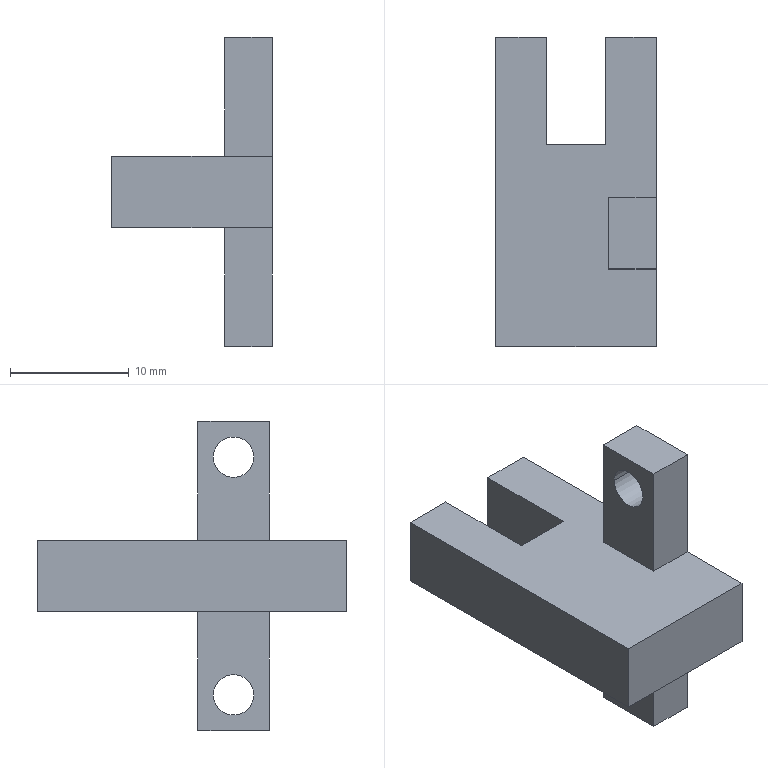Part | SolidWorks | features Extrusion 1, ICE 1 | 1 solid | 22 faces | box 13.5 x 26 x 26 mm | volume 2243 mm3 | plane 18 | cylinder 4 | commonest cylinder face diameters 3.4 x4
STEP:
#1=CARTESIAN_POINT('',(9.5,-18.2,10.));
#2=VERTEX_POINT('',#1);
#3=CARTESIAN_POINT('',(9.5,-14.8,10.));
#4=VERTEX_POINT('',#3);
#5=CARTESIAN_POINT('',(9.5,-16.5,10.));
#6=DIRECTION('',(1.,0.,0.));
#7=DIRECTION('',(0.,1.,0.));
#8=AXIS2_PLACEMENT_3D('',#5,#6,#7);
#9=CIRCLE('',#8,1.7);
#10=EDGE_CURVE('',#2,#4,#9,.T.);
#11=ORIENTED_EDGE('',*,*,#10,.F.);
#12=CARTESIAN_POINT('',(13.5,-18.2,10.));
#13=VERTEX_POINT('',#12);
#14=CARTESIAN_POINT('',(9.5,-18.2,10.));
#15=DIRECTION('',(1.,0.,0.));
#16=VECTOR('',#15,1000.);
#17=LINE('',#14,#16);
#18=EDGE_CURVE('',#2,#13,#17,.T.);
#19=ORIENTED_EDGE('',*,*,#18,.T.);
#20=CARTESIAN_POINT('',(13.5,-14.8,10.));
#21=VERTEX_POINT('',#20);
#22=CARTESIAN_POINT('',(13.5,-16.5,10.));
#23=DIRECTION('',(1.,0.,0.));
#24=DIRECTION('',(0.,1.,0.));
#25=AXIS2_PLACEMENT_3D('',#22,#23,#24);
#26=CIRCLE('',#25,1.7);
#27=EDGE_CURVE('',#13,#21,#26,.T.);
#28=ORIENTED_EDGE('',*,*,#27,.T.);
#29=CARTESIAN_POINT('',(9.5,-14.8,10.));
#30=DIRECTION('',(1.,0.,0.));
#31=VECTOR('',#30,1000.);
#32=LINE('',#29,#31);
#33=EDGE_CURVE('',#4,#21,#32,.T.);
#34=ORIENTED_EDGE('',*,*,#33,.F.);
#35=EDGE_LOOP('',(#11,#19,#28,#34));
#36=FACE_OUTER_BOUND('',#35,.T.);
#37=CARTESIAN_POINT('',(9.5,-16.5,10.));
#38=DIRECTION('',(1.,0.,0.));
#39=DIRECTION('',(0.,1.,0.));
#40=AXIS2_PLACEMENT_3D('',#37,#38,#39);
#41=CYLINDRICAL_SURFACE('',#40,1.7);
#42=ADVANCED_FACE('',(#36),#41,.F.);
#43=CARTESIAN_POINT('',(9.5,-18.2,-10.));
#44=VERTEX_POINT('',#43);
#45=CARTESIAN_POINT('',(9.5,-14.8,-10.));
#46=VERTEX_POINT('',#45);
#47=CARTESIAN_POINT('',(9.5,-16.5,-10.));
#48=DIRECTION('',(1.,0.,0.));
#49=DIRECTION('',(0.,1.,0.));
#50=AXIS2_PLACEMENT_3D('',#47,#48,#49);
#51=CIRCLE('',#50,1.7);
#52=EDGE_CURVE('',#44,#46,#51,.T.);
#53=ORIENTED_EDGE('',*,*,#52,.F.);
#54=CARTESIAN_POINT('',(13.5,-18.2,-10.));
#55=VERTEX_POINT('',#54);
#56=CARTESIAN_POINT('',(9.5,-18.2,-10.));
#57=DIRECTION('',(1.,0.,0.));
#58=VECTOR('',#57,1000.);
#59=LINE('',#56,#58);
#60=EDGE_CURVE('',#44,#55,#59,.T.);
#61=ORIENTED_EDGE('',*,*,#60,.T.);
#62=CARTESIAN_POINT('',(13.5,-14.8,-10.));
#63=VERTEX_POINT('',#62);
#64=CARTESIAN_POINT('',(13.5,-16.5,-10.));
#65=DIRECTION('',(1.,0.,0.));
#66=DIRECTION('',(0.,1.,0.));
#67=AXIS2_PLACEMENT_3D('',#64,#65,#66);
#68=CIRCLE('',#67,1.7);
#69=EDGE_CURVE('',#55,#63,#68,.T.);
#70=ORIENTED_EDGE('',*,*,#69,.T.);
#71=CARTESIAN_POINT('',(9.5,-14.8,-10.));
#72=DIRECTION('',(1.,0.,0.));
#73=VECTOR('',#72,1000.);
#74=LINE('',#71,#73);
#75=EDGE_CURVE('',#46,#63,#74,.T.);
#76=ORIENTED_EDGE('',*,*,#75,.F.);
#77=EDGE_LOOP('',(#53,#61,#70,#76));
#78=FACE_OUTER_BOUND('',#77,.T.);
#79=CARTESIAN_POINT('',(9.5,-16.5,-10.));
#80=DIRECTION('',(1.,0.,0.));
#81=DIRECTION('',(0.,1.,0.));
#82=AXIS2_PLACEMENT_3D('',#79,#80,#81);
#83=CYLINDRICAL_SURFACE('',#82,1.7);
#84=ADVANCED_FACE('',(#78),#83,.F.);
#85=CARTESIAN_POINT('',(0.,0.,-3.));
#86=VERTEX_POINT('',#85);
#87=CARTESIAN_POINT('',(0.,-26.,-3.));
#88=VERTEX_POINT('',#87);
#89=CARTESIAN_POINT('',(0.,0.,-3.));
#90=DIRECTION('',(0.,-1.,0.));
#91=VECTOR('',#90,1000.);
#92=LINE('',#89,#91);
#93=EDGE_CURVE('',#86,#88,#92,.T.);
#94=ORIENTED_EDGE('',*,*,#93,.T.);
#95=CARTESIAN_POINT('',(0.,-26.,3.));
#96=VERTEX_POINT('',#95);
#97=CARTESIAN_POINT('',(0.,-26.,3.));
#98=DIRECTION('',(0.,0.,-1.));
#99=VECTOR('',#98,1000.);
#100=LINE('',#97,#99);
#101=EDGE_CURVE('',#96,#88,#100,.T.);
#102=ORIENTED_EDGE('',*,*,#101,.F.);
#103=CARTESIAN_POINT('',(0.,0.,3.));
#104=VERTEX_POINT('',#103);
#105=CARTESIAN_POINT('',(0.,0.,3.));
#106=DIRECTION('',(0.,-1.,0.));
#107=VECTOR('',#106,1000.);
#108=LINE('',#105,#107);
#109=EDGE_CURVE('',#104,#96,#108,.T.);
#110=ORIENTED_EDGE('',*,*,#109,.F.);
#111=CARTESIAN_POINT('',(0.,0.,3.));
#112=DIRECTION('',(0.,0.,-1.));
#113=VECTOR('',#112,1000.);
#114=LINE('',#111,#113);
#115=EDGE_CURVE('',#104,#86,#114,.T.);
#116=ORIENTED_EDGE('',*,*,#115,.T.);
#117=EDGE_LOOP('',(#94,#102,#110,#116));
#118=FACE_OUTER_BOUND('',#117,.T.);
#119=CARTESIAN_POINT('',(0.,0.,3.));
#120=DIRECTION('',(1.,0.,0.));
#121=DIRECTION('',(0.,1.,0.));
#122=AXIS2_PLACEMENT_3D('',#119,#120,#121);
#123=PLANE('',#122);
#124=ADVANCED_FACE('',(#118),#123,.F.);
#125=CARTESIAN_POINT('',(13.5,-26.,-3.));
#126=VERTEX_POINT('',#125);
#127=CARTESIAN_POINT('',(0.,-26.,-3.));
#128=DIRECTION('',(1.,0.,0.));
#129=VECTOR('',#128,1000.);
#130=LINE('',#127,#129);
#131=EDGE_CURVE('',#88,#126,#130,.T.);
#132=ORIENTED_EDGE('',*,*,#131,.T.);
#133=CARTESIAN_POINT('',(13.5,-26.,3.));
#134=VERTEX_POINT('',#133);
#135=CARTESIAN_POINT('',(13.5,-26.,3.));
#136=DIRECTION('',(0.,0.,-1.));
#137=VECTOR('',#136,1000.);
#138=LINE('',#135,#137);
#139=EDGE_CURVE('',#134,#126,#138,.T.);
#140=ORIENTED_EDGE('',*,*,#139,.F.);
#141=CARTESIAN_POINT('',(0.,-26.,3.));
#142=DIRECTION('',(1.,0.,0.));
#143=VECTOR('',#142,1000.);
#144=LINE('',#141,#143);
#145=EDGE_CURVE('',#96,#134,#144,.T.);
#146=ORIENTED_EDGE('',*,*,#145,.F.);
#147=ORIENTED_EDGE('',*,*,#101,.T.);
#148=EDGE_LOOP('',(#132,#140,#146,#147));
#149=FACE_OUTER_BOUND('',#148,.T.);
#150=CARTESIAN_POINT('',(0.,-26.,3.));
#151=DIRECTION('',(0.,1.,0.));
#152=DIRECTION('',(0.,0.,1.));
#153=AXIS2_PLACEMENT_3D('',#150,#151,#152);
#154=PLANE('',#153);
#155=ADVANCED_FACE('',(#149),#154,.F.);
#156=CARTESIAN_POINT('',(13.5,-19.5,-3.));
#157=VERTEX_POINT('',#156);
#158=CARTESIAN_POINT('',(13.5,0.,-3.));
#159=DIRECTION('',(0.,1.,0.));
#160=VECTOR('',#159,1000.);
#161=LINE('',#158,#160);
#162=EDGE_CURVE('',#126,#157,#161,.T.);
#163=ORIENTED_EDGE('',*,*,#162,.T.);
#164=CARTESIAN_POINT('',(13.5,-19.5,-13.));
#165=VERTEX_POINT('',#164);
#166=CARTESIAN_POINT('',(13.5,-19.5,13.));
#167=DIRECTION('',(0.,0.,-1.));
#168=VECTOR('',#167,1000.);
#169=LINE('',#166,#168);
#170=EDGE_CURVE('',#157,#165,#169,.T.);
#171=ORIENTED_EDGE('',*,*,#170,.T.);
#172=CARTESIAN_POINT('',(13.5,-13.5,-13.));
#173=VERTEX_POINT('',#172);
#174=CARTESIAN_POINT('',(13.5,-13.5,-13.));
#175=DIRECTION('',(0.,1.,0.));
#176=VECTOR('',#175,1000.);
#177=LINE('',#174,#176);
#178=EDGE_CURVE('',#165,#173,#177,.T.);
#179=ORIENTED_EDGE('',*,*,#178,.T.);
#180=CARTESIAN_POINT('',(13.5,-13.5,-3.));
#181=VERTEX_POINT('',#180);
#182=CARTESIAN_POINT('',(13.5,-13.5,13.));
#183=DIRECTION('',(0.,0.,1.));
#184=VECTOR('',#183,1000.);
#185=LINE('',#182,#184);
#186=EDGE_CURVE('',#173,#181,#185,.T.);
#187=ORIENTED_EDGE('',*,*,#186,.T.);
#188=CARTESIAN_POINT('',(13.5,0.,-3.));
#189=VERTEX_POINT('',#188);
#190=CARTESIAN_POINT('',(13.5,0.,-3.));
#191=DIRECTION('',(0.,1.,0.));
#192=VECTOR('',#191,1000.);
#193=LINE('',#190,#192);
#194=EDGE_CURVE('',#181,#189,#193,.T.);
#195=ORIENTED_EDGE('',*,*,#194,.T.);
#196=CARTESIAN_POINT('',(13.5,0.,3.));
#197=VERTEX_POINT('',#196);
#198=CARTESIAN_POINT('',(13.5,0.,3.));
#199=DIRECTION('',(0.,0.,-1.));
#200=VECTOR('',#199,1000.);
#201=LINE('',#198,#200);
#202=EDGE_CURVE('',#197,#189,#201,.T.);
#203=ORIENTED_EDGE('',*,*,#202,.F.);
#204=CARTESIAN_POINT('',(13.5,-13.5,3.));
#205=VERTEX_POINT('',#204);
#206=CARTESIAN_POINT('',(13.5,0.,3.));
#207=DIRECTION('',(0.,1.,0.));
#208=VECTOR('',#207,1000.);
#209=LINE('',#206,#208);
#210=EDGE_CURVE('',#205,#197,#209,.T.);
#211=ORIENTED_EDGE('',*,*,#210,.F.);
#212=CARTESIAN_POINT('',(13.5,-13.5,13.));
#213=VERTEX_POINT('',#212);
#214=CARTESIAN_POINT('',(13.5,-13.5,13.));
#215=DIRECTION('',(0.,0.,1.));
#216=VECTOR('',#215,1000.);
#217=LINE('',#214,#216);
#218=EDGE_CURVE('',#205,#213,#217,.T.);
#219=ORIENTED_EDGE('',*,*,#218,.T.);
#220=CARTESIAN_POINT('',(13.5,-19.5,13.));
#221=VERTEX_POINT('',#220);
#222=CARTESIAN_POINT('',(13.5,-13.5,13.));
#223=DIRECTION('',(0.,-1.,0.));
#224=VECTOR('',#223,1000.);
#225=LINE('',#222,#224);
#226=EDGE_CURVE('',#213,#221,#225,.T.);
#227=ORIENTED_EDGE('',*,*,#226,.T.);
#228=CARTESIAN_POINT('',(13.5,-19.5,3.));
#229=VERTEX_POINT('',#228);
#230=CARTESIAN_POINT('',(13.5,-19.5,13.));
#231=DIRECTION('',(0.,0.,-1.));
#232=VECTOR('',#231,1000.);
#233=LINE('',#230,#232);
#234=EDGE_CURVE('',#221,#229,#233,.T.);
#235=ORIENTED_EDGE('',*,*,#234,.T.);
#236=CARTESIAN_POINT('',(13.5,0.,3.));
#237=DIRECTION('',(0.,1.,0.));
#238=VECTOR('',#237,1000.);
#239=LINE('',#236,#238);
#240=EDGE_CURVE('',#134,#229,#239,.T.);
#241=ORIENTED_EDGE('',*,*,#240,.F.);
#242=ORIENTED_EDGE('',*,*,#139,.T.);
#243=EDGE_LOOP('',(#163,#171,#179,#187,#195,#203,#211,#219,#227,#235,#241,#242));
#244=FACE_OUTER_BOUND('',#243,.T.);
#245=CARTESIAN_POINT('',(13.5,-16.5,-10.));
#246=DIRECTION('',(1.,0.,0.));
#247=DIRECTION('',(0.,1.,0.));
#248=AXIS2_PLACEMENT_3D('',#245,#246,#247);
#249=CIRCLE('',#248,1.7);
#250=EDGE_CURVE('',#63,#55,#249,.T.);
#251=ORIENTED_EDGE('',*,*,#250,.F.);
#252=ORIENTED_EDGE('',*,*,#69,.F.);
#253=EDGE_LOOP('',(#251,#252));
#254=FACE_BOUND('',#253,.T.);
#255=CARTESIAN_POINT('',(13.5,-16.5,10.));
#256=DIRECTION('',(1.,0.,0.));
#257=DIRECTION('',(0.,1.,0.));
#258=AXIS2_PLACEMENT_3D('',#255,#256,#257);
#259=CIRCLE('',#258,1.7);
#260=EDGE_CURVE('',#21,#13,#259,.T.);
#261=ORIENTED_EDGE('',*,*,#260,.F.);
#262=ORIENTED_EDGE('',*,*,#27,.F.);
#263=EDGE_LOOP('',(#261,#262));
#264=FACE_BOUND('',#263,.T.);
#265=CARTESIAN_POINT('',(13.5,0.,3.));
#266=DIRECTION('',(-1.,0.,0.));
#267=DIRECTION('',(0.,-1.,0.));
#268=AXIS2_PLACEMENT_3D('',#265,#266,#267);
#269=PLANE('',#268);
#270=ADVANCED_FACE('',(#244,#254,#264),#269,.F.);
#271=CARTESIAN_POINT('',(9.25,0.,-3.));
#272=VERTEX_POINT('',#271);
#273=CARTESIAN_POINT('',(9.25,0.,-3.));
#274=DIRECTION('',(-1.,0.,0.));
#275=VECTOR('',#274,1000.);
#276=LINE('',#273,#275);
#277=EDGE_CURVE('',#189,#272,#276,.T.);
#278=ORIENTED_EDGE('',*,*,#277,.T.);
#279=CARTESIAN_POINT('',(9.25,0.,3.));
#280=VERTEX_POINT('',#279);
#281=CARTESIAN_POINT('',(9.25,0.,3.));
#282=DIRECTION('',(0.,0.,-1.));
#283=VECTOR('',#282,1000.);
#284=LINE('',#281,#283);
#285=EDGE_CURVE('',#280,#272,#284,.T.);
#286=ORIENTED_EDGE('',*,*,#285,.F.);
#287=CARTESIAN_POINT('',(9.25,0.,3.));
#288=DIRECTION('',(-1.,0.,0.));
#289=VECTOR('',#288,1000.);
#290=LINE('',#287,#289);
#291=EDGE_CURVE('',#197,#280,#290,.T.);
#292=ORIENTED_EDGE('',*,*,#291,.F.);
#293=ORIENTED_EDGE('',*,*,#202,.T.);
#294=EDGE_LOOP('',(#278,#286,#292,#293));
#295=FACE_OUTER_BOUND('',#294,.T.);
#296=CARTESIAN_POINT('',(9.25,0.,3.));
#297=DIRECTION('',(0.,-1.,0.));
#298=DIRECTION('',(0.,0.,-1.));
#299=AXIS2_PLACEMENT_3D('',#296,#297,#298);
#300=PLANE('',#299);
#301=ADVANCED_FACE('',(#295),#300,.F.);
#302=CARTESIAN_POINT('',(9.25,-9.,-3.));
#303=VERTEX_POINT('',#302);
#304=CARTESIAN_POINT('',(9.25,0.,-3.));
#305=DIRECTION('',(0.,-1.,0.));
#306=VECTOR('',#305,1000.);
#307=LINE('',#304,#306);
#308=EDGE_CURVE('',#272,#303,#307,.T.);
#309=ORIENTED_EDGE('',*,*,#308,.T.);
#310=CARTESIAN_POINT('',(9.25,-9.,3.));
#311=VERTEX_POINT('',#310);
#312=CARTESIAN_POINT('',(9.25,-9.,3.));
#313=DIRECTION('',(0.,0.,-1.));
#314=VECTOR('',#313,1000.);
#315=LINE('',#312,#314);
#316=EDGE_CURVE('',#311,#303,#315,.T.);
#317=ORIENTED_EDGE('',*,*,#316,.F.);
#318=CARTESIAN_POINT('',(9.25,0.,3.));
#319=DIRECTION('',(0.,-1.,0.));
#320=VECTOR('',#319,1000.);
#321=LINE('',#318,#320);
#322=EDGE_CURVE('',#280,#311,#321,.T.);
#323=ORIENTED_EDGE('',*,*,#322,.F.);
#324=ORIENTED_EDGE('',*,*,#285,.T.);
#325=EDGE_LOOP('',(#309,#317,#323,#324));
#326=FACE_OUTER_BOUND('',#325,.T.);
#327=CARTESIAN_POINT('',(9.25,0.,3.));
#328=DIRECTION('',(1.,0.,0.));
#329=DIRECTION('',(0.,0.,-1.));
#330=AXIS2_PLACEMENT_3D('',#327,#328,#329);
#331=PLANE('',#330);
#332=ADVANCED_FACE('',(#326),#331,.F.);
#333=CARTESIAN_POINT('',(4.25,-9.,-3.));
#334=VERTEX_POINT('',#333);
#335=CARTESIAN_POINT('',(4.25,-9.,-3.));
#336=DIRECTION('',(-1.,0.,0.));
#337=VECTOR('',#336,1000.);
#338=LINE('',#335,#337);
#339=EDGE_CURVE('',#303,#334,#338,.T.);
#340=ORIENTED_EDGE('',*,*,#339,.T.);
#341=CARTESIAN_POINT('',(4.25,-9.,3.));
#342=VERTEX_POINT('',#341);
#343=CARTESIAN_POINT('',(4.25,-9.,3.));
#344=DIRECTION('',(0.,0.,-1.));
#345=VECTOR('',#344,1000.);
#346=LINE('',#343,#345);
#347=EDGE_CURVE('',#342,#334,#346,.T.);
#348=ORIENTED_EDGE('',*,*,#347,.F.);
#349=CARTESIAN_POINT('',(4.25,-9.,3.));
#350=DIRECTION('',(-1.,0.,0.));
#351=VECTOR('',#350,1000.);
#352=LINE('',#349,#351);
#353=EDGE_CURVE('',#311,#342,#352,.T.);
#354=ORIENTED_EDGE('',*,*,#353,.F.);
#355=ORIENTED_EDGE('',*,*,#316,.T.);
#356=EDGE_LOOP('',(#340,#348,#354,#355));
#357=FACE_OUTER_BOUND('',#356,.T.);
#358=CARTESIAN_POINT('',(4.25,-9.,3.));
#359=DIRECTION('',(0.,-1.,0.));
#360=DIRECTION('',(0.,0.,-1.));
#361=AXIS2_PLACEMENT_3D('',#358,#359,#360);
#362=PLANE('',#361);
#363=ADVANCED_FACE('',(#357),#362,.F.);
#364=CARTESIAN_POINT('',(4.25,0.,-3.));
#365=VERTEX_POINT('',#364);
#366=CARTESIAN_POINT('',(4.25,0.,-3.));
#367=DIRECTION('',(0.,1.,0.));
#368=VECTOR('',#367,1000.);
#369=LINE('',#366,#368);
#370=EDGE_CURVE('',#334,#365,#369,.T.);
#371=ORIENTED_EDGE('',*,*,#370,.T.);
#372=CARTESIAN_POINT('',(4.25,0.,3.));
#373=VERTEX_POINT('',#372);
#374=CARTESIAN_POINT('',(4.25,0.,3.));
#375=DIRECTION('',(0.,0.,-1.));
#376=VECTOR('',#375,1000.);
#377=LINE('',#374,#376);
#378=EDGE_CURVE('',#373,#365,#377,.T.);
#379=ORIENTED_EDGE('',*,*,#378,.F.);
#380=CARTESIAN_POINT('',(4.25,0.,3.));
#381=DIRECTION('',(0.,1.,0.));
#382=VECTOR('',#381,1000.);
#383=LINE('',#380,#382);
#384=EDGE_CURVE('',#342,#373,#383,.T.);
#385=ORIENTED_EDGE('',*,*,#384,.F.);
#386=ORIENTED_EDGE('',*,*,#347,.T.);
#387=EDGE_LOOP('',(#371,#379,#385,#386));
#388=FACE_OUTER_BOUND('',#387,.T.);
#389=CARTESIAN_POINT('',(4.25,0.,3.));
#390=DIRECTION('',(-1.,0.,0.));
#391=DIRECTION('',(0.,-1.,0.));
#392=AXIS2_PLACEMENT_3D('',#389,#390,#391);
#393=PLANE('',#392);
#394=ADVANCED_FACE('',(#388),#393,.F.);
#395=CARTESIAN_POINT('',(0.,0.,-3.));
#396=DIRECTION('',(-1.,0.,0.));
#397=VECTOR('',#396,1000.);
#398=LINE('',#395,#397);
#399=EDGE_CURVE('',#365,#86,#398,.T.);
#400=ORIENTED_EDGE('',*,*,#399,.T.);
#401=ORIENTED_EDGE('',*,*,#115,.F.);
#402=CARTESIAN_POINT('',(0.,0.,3.));
#403=DIRECTION('',(-1.,0.,0.));
#404=VECTOR('',#403,1000.);
#405=LINE('',#402,#404);
#406=EDGE_CURVE('',#373,#104,#405,.T.);
#407=ORIENTED_EDGE('',*,*,#406,.F.);
#408=ORIENTED_EDGE('',*,*,#378,.T.);
#409=EDGE_LOOP('',(#400,#401,#407,#408));
#410=FACE_OUTER_BOUND('',#409,.T.);
#411=CARTESIAN_POINT('',(0.,0.,3.));
#412=DIRECTION('',(0.,-1.,0.));
#413=DIRECTION('',(0.,0.,-1.));
#414=AXIS2_PLACEMENT_3D('',#411,#412,#413);
#415=PLANE('',#414);
#416=ADVANCED_FACE('',(#410),#415,.F.);
#417=CARTESIAN_POINT('',(9.5,-13.5,3.));
#418=VERTEX_POINT('',#417);
#419=CARTESIAN_POINT('',(0.,-13.5,3.));
#420=DIRECTION('',(-1.,0.,0.));
#421=VECTOR('',#420,1000.);
#422=LINE('',#419,#421);
#423=EDGE_CURVE('',#205,#418,#422,.T.);
#424=ORIENTED_EDGE('',*,*,#423,.F.);
#425=ORIENTED_EDGE('',*,*,#210,.T.);
#426=ORIENTED_EDGE('',*,*,#291,.T.);
#427=ORIENTED_EDGE('',*,*,#322,.T.);
#428=ORIENTED_EDGE('',*,*,#353,.T.);
#429=ORIENTED_EDGE('',*,*,#384,.T.);
#430=ORIENTED_EDGE('',*,*,#406,.T.);
#431=ORIENTED_EDGE('',*,*,#109,.T.);
#432=ORIENTED_EDGE('',*,*,#145,.T.);
#433=ORIENTED_EDGE('',*,*,#240,.T.);
#434=CARTESIAN_POINT('',(9.5,-19.5,3.));
#435=VERTEX_POINT('',#434);
#436=CARTESIAN_POINT('',(0.,-19.5,3.));
#437=DIRECTION('',(1.,0.,0.));
#438=VECTOR('',#437,1000.);
#439=LINE('',#436,#438);
#440=EDGE_CURVE('',#435,#229,#439,.T.);
#441=ORIENTED_EDGE('',*,*,#440,.F.);
#442=CARTESIAN_POINT('',(9.5,-26.,3.));
#443=DIRECTION('',(0.,1.,0.));
#444=VECTOR('',#443,1000.);
#445=LINE('',#442,#444);
#446=EDGE_CURVE('',#435,#418,#445,.T.);
#447=ORIENTED_EDGE('',*,*,#446,.T.);
#448=EDGE_LOOP('',(#424,#425,#426,#427,#428,#429,#430,#431,#432,#433,#441,#447));
#449=FACE_OUTER_BOUND('',#448,.T.);
#450=CARTESIAN_POINT('',(0.,-26.,3.));
#451=DIRECTION('',(0.,0.,1.));
#452=DIRECTION('',(1.,0.,0.));
#453=AXIS2_PLACEMENT_3D('',#450,#451,#452);
#454=PLANE('',#453);
#455=ADVANCED_FACE('',(#449),#454,.T.);
#456=ORIENTED_EDGE('',*,*,#194,.F.);
#457=CARTESIAN_POINT('',(9.5,-13.5,-3.));
#458=VERTEX_POINT('',#457);
#459=CARTESIAN_POINT('',(0.,-13.5,-3.));
#460=DIRECTION('',(-1.,0.,0.));
#461=VECTOR('',#460,1000.);
#462=LINE('',#459,#461);
#463=EDGE_CURVE('',#181,#458,#462,.T.);
#464=ORIENTED_EDGE('',*,*,#463,.T.);
#465=CARTESIAN_POINT('',(9.5,-19.5,-3.));
#466=VERTEX_POINT('',#465);
#467=CARTESIAN_POINT('',(9.5,-26.,-3.));
#468=DIRECTION('',(0.,1.,0.));
#469=VECTOR('',#468,1000.);
#470=LINE('',#467,#469);
#471=EDGE_CURVE('',#466,#458,#470,.T.);
#472=ORIENTED_EDGE('',*,*,#471,.F.);
#473=CARTESIAN_POINT('',(0.,-19.5,-3.));
#474=DIRECTION('',(1.,0.,0.));
#475=VECTOR('',#474,1000.);
#476=LINE('',#473,#475);
#477=EDGE_CURVE('',#466,#157,#476,.T.);
#478=ORIENTED_EDGE('',*,*,#477,.T.);
#479=ORIENTED_EDGE('',*,*,#162,.F.);
#480=ORIENTED_EDGE('',*,*,#131,.F.);
#481=ORIENTED_EDGE('',*,*,#93,.F.);
#482=ORIENTED_EDGE('',*,*,#399,.F.);
#483=ORIENTED_EDGE('',*,*,#370,.F.);
#484=ORIENTED_EDGE('',*,*,#339,.F.);
#485=ORIENTED_EDGE('',*,*,#308,.F.);
#486=ORIENTED_EDGE('',*,*,#277,.F.);
#487=EDGE_LOOP('',(#456,#464,#472,#478,#479,#480,#481,#482,#483,#484,#485,#486));
#488=FACE_OUTER_BOUND('',#487,.T.);
#489=CARTESIAN_POINT('',(0.,-26.,-3.));
#490=DIRECTION('',(0.,0.,1.));
#491=DIRECTION('',(1.,0.,0.));
#492=AXIS2_PLACEMENT_3D('',#489,#490,#491);
#493=PLANE('',#492);
#494=ADVANCED_FACE('',(#488),#493,.F.);
#495=ORIENTED_EDGE('',*,*,#178,.F.);
#496=CARTESIAN_POINT('',(9.5,-19.5,-13.));
#497=VERTEX_POINT('',#496);
#498=CARTESIAN_POINT('',(9.5,-19.5,-13.));
#499=DIRECTION('',(1.,0.,0.));
#500=VECTOR('',#499,1000.);
#501=LINE('',#498,#500);
#502=EDGE_CURVE('',#497,#165,#501,.T.);
#503=ORIENTED_EDGE('',*,*,#502,.F.);
#504=CARTESIAN_POINT('',(9.5,-13.5,-13.));
#505=VERTEX_POINT('',#504);
#506=CARTESIAN_POINT('',(9.5,-13.5,-13.));
#507=DIRECTION('',(0.,1.,0.));
#508=VECTOR('',#507,1000.);
#509=LINE('',#506,#508);
#510=EDGE_CURVE('',#497,#505,#509,.T.);
#511=ORIENTED_EDGE('',*,*,#510,.T.);
#512=CARTESIAN_POINT('',(9.5,-13.5,-13.));
#513=DIRECTION('',(1.,0.,0.));
#514=VECTOR('',#513,1000.);
#515=LINE('',#512,#514);
#516=EDGE_CURVE('',#505,#173,#515,.T.);
#517=ORIENTED_EDGE('',*,*,#516,.T.);
#518=EDGE_LOOP('',(#495,#503,#511,#517));
#519=FACE_OUTER_BOUND('',#518,.T.);
#520=CARTESIAN_POINT('',(9.5,-13.5,-13.));
#521=DIRECTION('',(0.,0.,-1.));
#522=DIRECTION('',(-1.,0.,0.));
#523=AXIS2_PLACEMENT_3D('',#520,#521,#522);
#524=PLANE('',#523);
#525=ADVANCED_FACE('',(#519),#524,.T.);
#526=ORIENTED_EDGE('',*,*,#60,.F.);
#527=CARTESIAN_POINT('',(9.5,-16.5,-10.));
#528=DIRECTION('',(1.,0.,0.));
#529=DIRECTION('',(0.,1.,0.));
#530=AXIS2_PLACEMENT_3D('',#527,#528,#529);
#531=CIRCLE('',#530,1.7);
#532=EDGE_CURVE('',#46,#44,#531,.T.);
#533=ORIENTED_EDGE('',*,*,#532,.F.);
#534=ORIENTED_EDGE('',*,*,#75,.T.);
#535=ORIENTED_EDGE('',*,*,#250,.T.);
#536=EDGE_LOOP('',(#526,#533,#534,#535));
#537=FACE_OUTER_BOUND('',#536,.T.);
#538=CARTESIAN_POINT('',(9.5,-16.5,-10.));
#539=DIRECTION('',(1.,0.,0.));
#540=DIRECTION('',(0.,1.,0.));
#541=AXIS2_PLACEMENT_3D('',#538,#539,#540);
#542=CYLINDRICAL_SURFACE('',#541,1.7);
#543=ADVANCED_FACE('',(#537),#542,.F.);
#544=ORIENTED_EDGE('',*,*,#532,.T.);
#545=ORIENTED_EDGE('',*,*,#52,.T.);
#546=EDGE_LOOP('',(#544,#545));
#547=FACE_BOUND('',#546,.T.);
#548=CARTESIAN_POINT('',(9.5,-19.5,13.));
#549=DIRECTION('',(0.,0.,-1.));
#550=VECTOR('',#549,1000.);
#551=LINE('',#548,#550);
#552=EDGE_CURVE('',#466,#497,#551,.T.);
#553=ORIENTED_EDGE('',*,*,#552,.F.);
#554=ORIENTED_EDGE('',*,*,#471,.T.);
#555=CARTESIAN_POINT('',(9.5,-13.5,13.));
#556=DIRECTION('',(0.,0.,1.));
#557=VECTOR('',#556,1000.);
#558=LINE('',#555,#557);
#559=EDGE_CURVE('',#505,#458,#558,.T.);
#560=ORIENTED_EDGE('',*,*,#559,.F.);
#561=ORIENTED_EDGE('',*,*,#510,.F.);
#562=EDGE_LOOP('',(#553,#554,#560,#561));
#563=FACE_OUTER_BOUND('',#562,.T.);
#564=CARTESIAN_POINT('',(9.5,-19.5,13.));
#565=DIRECTION('',(1.,0.,0.));
#566=DIRECTION('',(0.,1.,0.));
#567=AXIS2_PLACEMENT_3D('',#564,#565,#566);
#568=PLANE('',#567);
#569=ADVANCED_FACE('',(#547,#563),#568,.F.);
#570=ORIENTED_EDGE('',*,*,#477,.F.);
#571=ORIENTED_EDGE('',*,*,#552,.T.);
#572=ORIENTED_EDGE('',*,*,#502,.T.);
#573=ORIENTED_EDGE('',*,*,#170,.F.);
#574=EDGE_LOOP('',(#570,#571,#572,#573));
#575=FACE_OUTER_BOUND('',#574,.T.);
#576=CARTESIAN_POINT('',(9.5,-19.5,13.));
#577=DIRECTION('',(0.,-1.,0.));
#578=DIRECTION('',(1.,0.,0.));
#579=AXIS2_PLACEMENT_3D('',#576,#577,#578);
#580=PLANE('',#579);
#581=ADVANCED_FACE('',(#575),#580,.T.);
#582=ORIENTED_EDGE('',*,*,#463,.F.);
#583=ORIENTED_EDGE('',*,*,#186,.F.);
#584=ORIENTED_EDGE('',*,*,#516,.F.);
#585=ORIENTED_EDGE('',*,*,#559,.T.);
#586=EDGE_LOOP('',(#582,#583,#584,#585));
#587=FACE_OUTER_BOUND('',#586,.T.);
#588=CARTESIAN_POINT('',(9.5,-13.5,13.));
#589=DIRECTION('',(0.,1.,0.));
#590=DIRECTION('',(-1.,0.,0.));
#591=AXIS2_PLACEMENT_3D('',#588,#589,#590);
#592=PLANE('',#591);
#593=ADVANCED_FACE('',(#587),#592,.T.);
#594=ORIENTED_EDGE('',*,*,#226,.F.);
#595=CARTESIAN_POINT('',(9.5,-13.5,13.));
#596=VERTEX_POINT('',#595);
#597=CARTESIAN_POINT('',(9.5,-13.5,13.));
#598=DIRECTION('',(1.,0.,0.));
#599=VECTOR('',#598,1000.);
#600=LINE('',#597,#599);
#601=EDGE_CURVE('',#596,#213,#600,.T.);
#602=ORIENTED_EDGE('',*,*,#601,.F.);
#603=CARTESIAN_POINT('',(9.5,-19.5,13.));
#604=VERTEX_POINT('',#603);
#605=CARTESIAN_POINT('',(9.5,-13.5,13.));
#606=DIRECTION('',(0.,-1.,0.));
#607=VECTOR('',#606,1000.);
#608=LINE('',#605,#607);
#609=EDGE_CURVE('',#596,#604,#608,.T.);
#610=ORIENTED_EDGE('',*,*,#609,.T.);
#611=CARTESIAN_POINT('',(9.5,-19.5,13.));
#612=DIRECTION('',(1.,0.,0.));
#613=VECTOR('',#612,1000.);
#614=LINE('',#611,#613);
#615=EDGE_CURVE('',#604,#221,#614,.T.);
#616=ORIENTED_EDGE('',*,*,#615,.T.);
#617=EDGE_LOOP('',(#594,#602,#610,#616));
#618=FACE_OUTER_BOUND('',#617,.T.);
#619=CARTESIAN_POINT('',(9.5,-13.5,13.));
#620=DIRECTION('',(0.,0.,1.));
#621=DIRECTION('',(0.,-1.,0.));
#622=AXIS2_PLACEMENT_3D('',#619,#620,#621);
#623=PLANE('',#622);
#624=ADVANCED_FACE('',(#618),#623,.T.);
#625=ORIENTED_EDGE('',*,*,#218,.F.);
#626=ORIENTED_EDGE('',*,*,#423,.T.);
#627=CARTESIAN_POINT('',(9.5,-13.5,13.));
#628=DIRECTION('',(0.,0.,1.));
#629=VECTOR('',#628,1000.);
#630=LINE('',#627,#629);
#631=EDGE_CURVE('',#418,#596,#630,.T.);
#632=ORIENTED_EDGE('',*,*,#631,.T.);
#633=ORIENTED_EDGE('',*,*,#601,.T.);
#634=EDGE_LOOP('',(#625,#626,#632,#633));
#635=FACE_OUTER_BOUND('',#634,.T.);
#636=CARTESIAN_POINT('',(9.5,-13.5,13.));
#637=DIRECTION('',(0.,1.,0.));
#638=DIRECTION('',(-1.,0.,0.));
#639=AXIS2_PLACEMENT_3D('',#636,#637,#638);
#640=PLANE('',#639);
#641=ADVANCED_FACE('',(#635),#640,.T.);
#642=CARTESIAN_POINT('',(9.5,-19.5,13.));
#643=DIRECTION('',(0.,0.,-1.));
#644=VECTOR('',#643,1000.);
#645=LINE('',#642,#644);
#646=EDGE_CURVE('',#604,#435,#645,.T.);
#647=ORIENTED_EDGE('',*,*,#646,.T.);
#648=ORIENTED_EDGE('',*,*,#440,.T.);
#649=ORIENTED_EDGE('',*,*,#234,.F.);
#650=ORIENTED_EDGE('',*,*,#615,.F.);
#651=EDGE_LOOP('',(#647,#648,#649,#650));
#652=FACE_OUTER_BOUND('',#651,.T.);
#653=CARTESIAN_POINT('',(9.5,-19.5,13.));
#654=DIRECTION('',(0.,-1.,0.));
#655=DIRECTION('',(1.,0.,0.));
#656=AXIS2_PLACEMENT_3D('',#653,#654,#655);
#657=PLANE('',#656);
#658=ADVANCED_FACE('',(#652),#657,.T.);
#659=ORIENTED_EDGE('',*,*,#446,.F.);
#660=ORIENTED_EDGE('',*,*,#646,.F.);
#661=ORIENTED_EDGE('',*,*,#609,.F.);
#662=ORIENTED_EDGE('',*,*,#631,.F.);
#663=EDGE_LOOP('',(#659,#660,#661,#662));
#664=FACE_OUTER_BOUND('',#663,.T.);
#665=CARTESIAN_POINT('',(9.5,-16.5,10.));
#666=DIRECTION('',(1.,0.,0.));
#667=DIRECTION('',(0.,1.,0.));
#668=AXIS2_PLACEMENT_3D('',#665,#666,#667);
#669=CIRCLE('',#668,1.7);
#670=EDGE_CURVE('',#4,#2,#669,.T.);
#671=ORIENTED_EDGE('',*,*,#670,.T.);
#672=ORIENTED_EDGE('',*,*,#10,.T.);
#673=EDGE_LOOP('',(#671,#672));
#674=FACE_BOUND('',#673,.T.);
#675=CARTESIAN_POINT('',(9.5,-19.5,13.));
#676=DIRECTION('',(1.,0.,0.));
#677=DIRECTION('',(0.,1.,0.));
#678=AXIS2_PLACEMENT_3D('',#675,#676,#677);
#679=PLANE('',#678);
#680=ADVANCED_FACE('',(#664,#674),#679,.F.);
#681=ORIENTED_EDGE('',*,*,#18,.F.);
#682=ORIENTED_EDGE('',*,*,#670,.F.);
#683=ORIENTED_EDGE('',*,*,#33,.T.);
#684=ORIENTED_EDGE('',*,*,#260,.T.);
#685=EDGE_LOOP('',(#681,#682,#683,#684));
#686=FACE_OUTER_BOUND('',#685,.T.);
#687=CARTESIAN_POINT('',(9.5,-16.5,10.));
#688=DIRECTION('',(1.,0.,0.));
#689=DIRECTION('',(0.,1.,0.));
#690=AXIS2_PLACEMENT_3D('',#687,#688,#689);
#691=CYLINDRICAL_SURFACE('',#690,1.7);
#692=ADVANCED_FACE('',(#686),#691,.F.);
#693=CLOSED_SHELL('',(#42,#84,#124,#155,#270,#301,#332,#363,#394,#416,#455,#494,#525,#543,#569,#581,#593,#624,#641,#658,#680,#692));
#694=MANIFOLD_SOLID_BREP('',#693);
#695=CARTESIAN_POINT('',(0.,0.,0.));
#696=DIRECTION('',(0.,0.,1.));
#697=DIRECTION('',(1.,0.,0.));
#698=AXIS2_PLACEMENT_3D('',#695,#696,#697);
#699=(LENGTH_UNIT()NAMED_UNIT(*)SI_UNIT(.MILLI.,.METRE.));
#700=UNCERTAINTY_MEASURE_WITH_UNIT(LENGTH_MEASURE(0.00001),#699,'','');
#701=(NAMED_UNIT(*)PLANE_ANGLE_UNIT()SI_UNIT($,.RADIAN.));
#702=(NAMED_UNIT(*)SI_UNIT($,.STERADIAN.)SOLID_ANGLE_UNIT());
#703=(GEOMETRIC_REPRESENTATION_CONTEXT(3)GLOBAL_UNCERTAINTY_ASSIGNED_CONTEXT((#700))GLOBAL_UNIT_ASSIGNED_CONTEXT((#699,#701,#702))REPRESENTATION_CONTEXT('',''));
#704=ADVANCED_BREP_SHAPE_REPRESENTATION('',(#694,#698),#703);